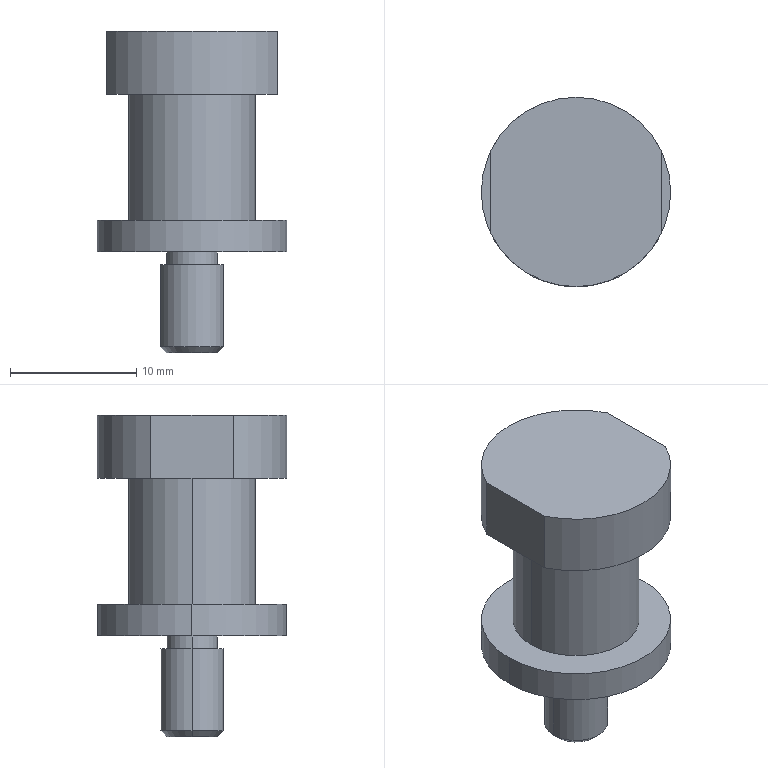Part | STEP file | PN_0036 | 1 solid | 20 faces | box 15 x 15 x 25.5 mm | volume 2226 mm3 | cylinder 10 | plane 8 | cone 2 | commonest cylinder face diameters 15 x4 4 x2 5 x2 10 x2
STEP:
#1=CARTESIAN_POINT('',(0.,0.,0.));
#2=DIRECTION('',(0.,0.,1.));
#3=DIRECTION('',(1.,0.,0.));
#4=AXIS2_PLACEMENT_3D('',#1,#2,#3);
#5=CARTESIAN_POINT('',(-2.,0.,-10.5));
#6=VERTEX_POINT('',#5);
#7=CARTESIAN_POINT('',(2.,0.,-10.5));
#8=VERTEX_POINT('',#7);
#9=CARTESIAN_POINT('',(0.,0.,-10.5));
#10=DIRECTION('',(0.,0.,-1.));
#11=DIRECTION('',(-1.,0.,0.));
#12=AXIS2_PLACEMENT_3D('',#9,#10,#11);
#13=CIRCLE('',#12,2.);
#14=CARTESIAN_POINT('',(0.,0.,-10.5));
#15=DIRECTION('',(0.,0.,1.));
#16=DIRECTION('',(1.,0.,0.));
#17=AXIS2_PLACEMENT_3D('',#14,#15,#16);
#18=CONICAL_SURFACE('',#17,2.,0.7854);
#19=CARTESIAN_POINT('',(3.142,0.));
#20=DIRECTION('',(-1.,0.));
#21=VECTOR('',#20,1.);
#22=LINE('',#19,#21);
#23=(GEOMETRIC_REPRESENTATION_CONTEXT(2)PARAMETRIC_REPRESENTATION_CONTEXT()REPRESENTATION_CONTEXT('',''));
#24=DEFINITIONAL_REPRESENTATION('',(#22),#23);
#25=PCURVE('',#18,#24);
#26=CARTESIAN_POINT('',(0.,0.,-10.5));
#27=DIRECTION('',(0.,0.,-1.));
#28=DIRECTION('',(-1.,0.,0.));
#29=AXIS2_PLACEMENT_3D('',#26,#27,#28);
#30=PLANE('',#29);
#31=CARTESIAN_POINT('',(0.,0.));
#32=DIRECTION('',(1.,0.));
#33=AXIS2_PLACEMENT_2D('',#31,#32);
#34=CIRCLE('',#33,2.);
#35=(GEOMETRIC_REPRESENTATION_CONTEXT(2)PARAMETRIC_REPRESENTATION_CONTEXT()REPRESENTATION_CONTEXT('',''));
#36=DEFINITIONAL_REPRESENTATION('',(#34),#35);
#37=PCURVE('',#30,#36);
#38=SURFACE_CURVE('',#13,(#25,#37),.PCURVE_S1.);
#39=EDGE_CURVE('',#6,#8,#38,.T.);
#40=ORIENTED_EDGE('',*,*,#39,.F.);
#41=CARTESIAN_POINT('',(-2.5,0.,-10.));
#42=VERTEX_POINT('',#41);
#43=CARTESIAN_POINT('',(-2.,0.,-10.5));
#44=DIRECTION('',(-0.7071,0.,0.7071));
#45=VECTOR('',#44,1.);
#46=LINE('',#43,#45);
#47=CARTESIAN_POINT('',(3.142,0.));
#48=DIRECTION('',(0.,1.));
#49=VECTOR('',#48,1.);
#50=LINE('',#47,#49);
#51=(GEOMETRIC_REPRESENTATION_CONTEXT(2)PARAMETRIC_REPRESENTATION_CONTEXT()REPRESENTATION_CONTEXT('',''));
#52=DEFINITIONAL_REPRESENTATION('',(#50),#51);
#53=PCURVE('',#18,#52);
#54=CARTESIAN_POINT('',(0.,0.,-10.5));
#55=DIRECTION('',(0.,0.,1.));
#56=DIRECTION('',(1.,0.,0.));
#57=AXIS2_PLACEMENT_3D('',#54,#55,#56);
#58=CONICAL_SURFACE('',#57,2.,0.7854);
#59=CARTESIAN_POINT('',(3.142,0.));
#60=DIRECTION('',(0.,1.));
#61=VECTOR('',#60,1.);
#62=LINE('',#59,#61);
#63=(GEOMETRIC_REPRESENTATION_CONTEXT(2)PARAMETRIC_REPRESENTATION_CONTEXT()REPRESENTATION_CONTEXT('',''));
#64=DEFINITIONAL_REPRESENTATION('',(#62),#63);
#65=PCURVE('',#58,#64);
#66=SURFACE_CURVE('',#46,(#53,#65),.PCURVE_S1.);
#67=EDGE_CURVE('',#6,#42,#66,.T.);
#68=ORIENTED_EDGE('',*,*,#67,.T.);
#69=CARTESIAN_POINT('',(2.5,0.,-10.));
#70=VERTEX_POINT('',#69);
#71=CARTESIAN_POINT('',(0.,0.,-10.));
#72=DIRECTION('',(0.,0.,1.));
#73=DIRECTION('',(-1.,0.,0.));
#74=AXIS2_PLACEMENT_3D('',#71,#72,#73);
#75=CIRCLE('',#74,2.5);
#76=CARTESIAN_POINT('',(-3.142,0.5));
#77=DIRECTION('',(1.,0.));
#78=VECTOR('',#77,1.);
#79=LINE('',#76,#78);
#80=(GEOMETRIC_REPRESENTATION_CONTEXT(2)PARAMETRIC_REPRESENTATION_CONTEXT()REPRESENTATION_CONTEXT('',''));
#81=DEFINITIONAL_REPRESENTATION('',(#79),#80);
#82=PCURVE('',#18,#81);
#83=CARTESIAN_POINT('',(0.,0.,-10.5));
#84=DIRECTION('',(0.,0.,1.));
#85=DIRECTION('',(1.,0.,0.));
#86=AXIS2_PLACEMENT_3D('',#83,#84,#85);
#87=CYLINDRICAL_SURFACE('',#86,2.5);
#88=CARTESIAN_POINT('',(-3.142,0.5));
#89=DIRECTION('',(1.,0.));
#90=VECTOR('',#89,1.);
#91=LINE('',#88,#90);
#92=(GEOMETRIC_REPRESENTATION_CONTEXT(2)PARAMETRIC_REPRESENTATION_CONTEXT()REPRESENTATION_CONTEXT('',''));
#93=DEFINITIONAL_REPRESENTATION('',(#91),#92);
#94=PCURVE('',#87,#93);
#95=SURFACE_CURVE('',#75,(#82,#94),.PCURVE_S1.);
#96=EDGE_CURVE('',#70,#42,#95,.T.);
#97=ORIENTED_EDGE('',*,*,#96,.F.);
#98=CARTESIAN_POINT('',(2.,0.,-10.5));
#99=DIRECTION('',(0.7071,0.,0.7071));
#100=VECTOR('',#99,1.);
#101=LINE('',#98,#100);
#102=CARTESIAN_POINT('',(0.,0.));
#103=DIRECTION('',(0.,1.));
#104=VECTOR('',#103,1.);
#105=LINE('',#102,#104);
#106=(GEOMETRIC_REPRESENTATION_CONTEXT(2)PARAMETRIC_REPRESENTATION_CONTEXT()REPRESENTATION_CONTEXT('',''));
#107=DEFINITIONAL_REPRESENTATION('',(#105),#106);
#108=PCURVE('',#18,#107);
#109=CARTESIAN_POINT('',(6.283,0.));
#110=DIRECTION('',(0.,1.));
#111=VECTOR('',#110,1.);
#112=LINE('',#109,#111);
#113=(GEOMETRIC_REPRESENTATION_CONTEXT(2)PARAMETRIC_REPRESENTATION_CONTEXT()REPRESENTATION_CONTEXT('',''));
#114=DEFINITIONAL_REPRESENTATION('',(#112),#113);
#115=PCURVE('',#58,#114);
#116=SURFACE_CURVE('',#101,(#108,#115),.PCURVE_S1.);
#117=EDGE_CURVE('',#8,#70,#116,.T.);
#118=ORIENTED_EDGE('',*,*,#117,.F.);
#119=EDGE_LOOP('',(#40,#68,#97,#118));
#120=FACE_BOUND('',#119,.T.);
#121=ADVANCED_FACE('',(#120),#18,.T.);
#122=ORIENTED_EDGE('',*,*,#96,.T.);
#123=CARTESIAN_POINT('',(-2.5,0.,-3.5));
#124=VERTEX_POINT('',#123);
#125=CARTESIAN_POINT('',(-2.5,0.,-10.5));
#126=DIRECTION('',(0.,0.,1.));
#127=VECTOR('',#126,1.);
#128=LINE('',#125,#127);
#129=CARTESIAN_POINT('',(3.142,0.));
#130=DIRECTION('',(0.,1.));
#131=VECTOR('',#130,1.);
#132=LINE('',#129,#131);
#133=(GEOMETRIC_REPRESENTATION_CONTEXT(2)PARAMETRIC_REPRESENTATION_CONTEXT()REPRESENTATION_CONTEXT('',''));
#134=DEFINITIONAL_REPRESENTATION('',(#132),#133);
#135=PCURVE('',#87,#134);
#136=CARTESIAN_POINT('',(0.,0.,-10.5));
#137=DIRECTION('',(0.,0.,1.));
#138=DIRECTION('',(1.,0.,0.));
#139=AXIS2_PLACEMENT_3D('',#136,#137,#138);
#140=CYLINDRICAL_SURFACE('',#139,2.5);
#141=CARTESIAN_POINT('',(3.142,0.));
#142=DIRECTION('',(0.,1.));
#143=VECTOR('',#142,1.);
#144=LINE('',#141,#143);
#145=(GEOMETRIC_REPRESENTATION_CONTEXT(2)PARAMETRIC_REPRESENTATION_CONTEXT()REPRESENTATION_CONTEXT('',''));
#146=DEFINITIONAL_REPRESENTATION('',(#144),#145);
#147=PCURVE('',#140,#146);
#148=SURFACE_CURVE('',#128,(#135,#147),.PCURVE_S1.);
#149=EDGE_CURVE('',#42,#124,#148,.T.);
#150=ORIENTED_EDGE('',*,*,#149,.T.);
#151=CARTESIAN_POINT('',(2.5,0.,-3.5));
#152=VERTEX_POINT('',#151);
#153=CARTESIAN_POINT('',(0.,0.,-3.5));
#154=DIRECTION('',(0.,0.,-1.));
#155=DIRECTION('',(-1.,0.,0.));
#156=AXIS2_PLACEMENT_3D('',#153,#154,#155);
#157=CIRCLE('',#156,2.5);
#158=CARTESIAN_POINT('',(3.142,7.));
#159=DIRECTION('',(-1.,0.));
#160=VECTOR('',#159,1.);
#161=LINE('',#158,#160);
#162=(GEOMETRIC_REPRESENTATION_CONTEXT(2)PARAMETRIC_REPRESENTATION_CONTEXT()REPRESENTATION_CONTEXT('',''));
#163=DEFINITIONAL_REPRESENTATION('',(#161),#162);
#164=PCURVE('',#87,#163);
#165=CARTESIAN_POINT('',(0.,0.,-3.5));
#166=DIRECTION('',(0.,0.,-1.));
#167=DIRECTION('',(-1.,0.,0.));
#168=AXIS2_PLACEMENT_3D('',#165,#166,#167);
#169=PLANE('',#168);
#170=CARTESIAN_POINT('',(0.,0.));
#171=DIRECTION('',(1.,0.));
#172=AXIS2_PLACEMENT_2D('',#170,#171);
#173=CIRCLE('',#172,2.5);
#174=(GEOMETRIC_REPRESENTATION_CONTEXT(2)PARAMETRIC_REPRESENTATION_CONTEXT()REPRESENTATION_CONTEXT('',''));
#175=DEFINITIONAL_REPRESENTATION('',(#173),#174);
#176=PCURVE('',#169,#175);
#177=SURFACE_CURVE('',#157,(#164,#176),.PCURVE_S1.);
#178=EDGE_CURVE('',#124,#152,#177,.T.);
#179=ORIENTED_EDGE('',*,*,#178,.T.);
#180=CARTESIAN_POINT('',(2.5,0.,-10.5));
#181=DIRECTION('',(0.,0.,1.));
#182=VECTOR('',#181,1.);
#183=LINE('',#180,#182);
#184=CARTESIAN_POINT('',(0.,0.));
#185=DIRECTION('',(0.,1.));
#186=VECTOR('',#185,1.);
#187=LINE('',#184,#186);
#188=(GEOMETRIC_REPRESENTATION_CONTEXT(2)PARAMETRIC_REPRESENTATION_CONTEXT()REPRESENTATION_CONTEXT('',''));
#189=DEFINITIONAL_REPRESENTATION('',(#187),#188);
#190=PCURVE('',#87,#189);
#191=CARTESIAN_POINT('',(6.283,0.));
#192=DIRECTION('',(0.,1.));
#193=VECTOR('',#192,1.);
#194=LINE('',#191,#193);
#195=(GEOMETRIC_REPRESENTATION_CONTEXT(2)PARAMETRIC_REPRESENTATION_CONTEXT()REPRESENTATION_CONTEXT('',''));
#196=DEFINITIONAL_REPRESENTATION('',(#194),#195);
#197=PCURVE('',#140,#196);
#198=SURFACE_CURVE('',#183,(#190,#197),.PCURVE_S1.);
#199=EDGE_CURVE('',#70,#152,#198,.T.);
#200=ORIENTED_EDGE('',*,*,#199,.F.);
#201=EDGE_LOOP('',(#122,#150,#179,#200));
#202=FACE_BOUND('',#201,.T.);
#203=ADVANCED_FACE('',(#202),#87,.T.);
#204=CARTESIAN_POINT('',(-2.,0.,-3.5));
#205=VERTEX_POINT('',#204);
#206=CARTESIAN_POINT('',(2.,0.,-3.5));
#207=VERTEX_POINT('',#206);
#208=CARTESIAN_POINT('',(0.,0.,-3.5));
#209=DIRECTION('',(0.,0.,-1.));
#210=DIRECTION('',(-1.,0.,0.));
#211=AXIS2_PLACEMENT_3D('',#208,#209,#210);
#212=CIRCLE('',#211,2.);
#213=CARTESIAN_POINT('',(0.,0.,-3.5));
#214=DIRECTION('',(0.,0.,1.));
#215=DIRECTION('',(1.,0.,0.));
#216=AXIS2_PLACEMENT_3D('',#213,#214,#215);
#217=CYLINDRICAL_SURFACE('',#216,2.);
#218=CARTESIAN_POINT('',(3.142,0.));
#219=DIRECTION('',(-1.,0.));
#220=VECTOR('',#219,1.);
#221=LINE('',#218,#220);
#222=(GEOMETRIC_REPRESENTATION_CONTEXT(2)PARAMETRIC_REPRESENTATION_CONTEXT()REPRESENTATION_CONTEXT('',''));
#223=DEFINITIONAL_REPRESENTATION('',(#221),#222);
#224=PCURVE('',#217,#223);
#225=CARTESIAN_POINT('',(0.,0.));
#226=DIRECTION('',(1.,0.));
#227=AXIS2_PLACEMENT_2D('',#225,#226);
#228=CIRCLE('',#227,2.);
#229=(GEOMETRIC_REPRESENTATION_CONTEXT(2)PARAMETRIC_REPRESENTATION_CONTEXT()REPRESENTATION_CONTEXT('',''));
#230=DEFINITIONAL_REPRESENTATION('',(#228),#229);
#231=PCURVE('',#169,#230);
#232=SURFACE_CURVE('',#212,(#224,#231),.PCURVE_S1.);
#233=EDGE_CURVE('',#205,#207,#232,.T.);
#234=ORIENTED_EDGE('',*,*,#233,.F.);
#235=CARTESIAN_POINT('',(-2.,0.,-2.5));
#236=VERTEX_POINT('',#235);
#237=CARTESIAN_POINT('',(-2.,0.,-3.5));
#238=DIRECTION('',(0.,0.,1.));
#239=VECTOR('',#238,1.);
#240=LINE('',#237,#239);
#241=CARTESIAN_POINT('',(3.142,0.));
#242=DIRECTION('',(0.,1.));
#243=VECTOR('',#242,1.);
#244=LINE('',#241,#243);
#245=(GEOMETRIC_REPRESENTATION_CONTEXT(2)PARAMETRIC_REPRESENTATION_CONTEXT()REPRESENTATION_CONTEXT('',''));
#246=DEFINITIONAL_REPRESENTATION('',(#244),#245);
#247=PCURVE('',#217,#246);
#248=CARTESIAN_POINT('',(0.,0.,-3.5));
#249=DIRECTION('',(0.,0.,1.));
#250=DIRECTION('',(1.,0.,0.));
#251=AXIS2_PLACEMENT_3D('',#248,#249,#250);
#252=CYLINDRICAL_SURFACE('',#251,2.);
#253=CARTESIAN_POINT('',(3.142,0.));
#254=DIRECTION('',(0.,1.));
#255=VECTOR('',#254,1.);
#256=LINE('',#253,#255);
#257=(GEOMETRIC_REPRESENTATION_CONTEXT(2)PARAMETRIC_REPRESENTATION_CONTEXT()REPRESENTATION_CONTEXT('',''));
#258=DEFINITIONAL_REPRESENTATION('',(#256),#257);
#259=PCURVE('',#252,#258);
#260=SURFACE_CURVE('',#240,(#247,#259),.PCURVE_S1.);
#261=EDGE_CURVE('',#205,#236,#260,.T.);
#262=ORIENTED_EDGE('',*,*,#261,.T.);
#263=CARTESIAN_POINT('',(2.,0.,-2.5));
#264=VERTEX_POINT('',#263);
#265=CARTESIAN_POINT('',(0.,0.,-2.5));
#266=DIRECTION('',(0.,0.,-1.));
#267=DIRECTION('',(-1.,0.,0.));
#268=AXIS2_PLACEMENT_3D('',#265,#266,#267);
#269=CIRCLE('',#268,2.);
#270=CARTESIAN_POINT('',(3.142,1.));
#271=DIRECTION('',(-1.,0.));
#272=VECTOR('',#271,1.);
#273=LINE('',#270,#272);
#274=(GEOMETRIC_REPRESENTATION_CONTEXT(2)PARAMETRIC_REPRESENTATION_CONTEXT()REPRESENTATION_CONTEXT('',''));
#275=DEFINITIONAL_REPRESENTATION('',(#273),#274);
#276=PCURVE('',#217,#275);
#277=CARTESIAN_POINT('',(0.,0.,-2.5));
#278=DIRECTION('',(0.,0.,-1.));
#279=DIRECTION('',(-1.,0.,0.));
#280=AXIS2_PLACEMENT_3D('',#277,#278,#279);
#281=PLANE('',#280);
#282=CARTESIAN_POINT('',(0.,0.));
#283=DIRECTION('',(1.,0.));
#284=AXIS2_PLACEMENT_2D('',#282,#283);
#285=CIRCLE('',#284,2.);
#286=(GEOMETRIC_REPRESENTATION_CONTEXT(2)PARAMETRIC_REPRESENTATION_CONTEXT()REPRESENTATION_CONTEXT('',''));
#287=DEFINITIONAL_REPRESENTATION('',(#285),#286);
#288=PCURVE('',#281,#287);
#289=SURFACE_CURVE('',#269,(#276,#288),.PCURVE_S1.);
#290=EDGE_CURVE('',#236,#264,#289,.T.);
#291=ORIENTED_EDGE('',*,*,#290,.T.);
#292=CARTESIAN_POINT('',(2.,0.,-3.5));
#293=DIRECTION('',(0.,0.,1.));
#294=VECTOR('',#293,1.);
#295=LINE('',#292,#294);
#296=CARTESIAN_POINT('',(0.,0.));
#297=DIRECTION('',(0.,1.));
#298=VECTOR('',#297,1.);
#299=LINE('',#296,#298);
#300=(GEOMETRIC_REPRESENTATION_CONTEXT(2)PARAMETRIC_REPRESENTATION_CONTEXT()REPRESENTATION_CONTEXT('',''));
#301=DEFINITIONAL_REPRESENTATION('',(#299),#300);
#302=PCURVE('',#217,#301);
#303=CARTESIAN_POINT('',(6.283,0.));
#304=DIRECTION('',(0.,1.));
#305=VECTOR('',#304,1.);
#306=LINE('',#303,#305);
#307=(GEOMETRIC_REPRESENTATION_CONTEXT(2)PARAMETRIC_REPRESENTATION_CONTEXT()REPRESENTATION_CONTEXT('',''));
#308=DEFINITIONAL_REPRESENTATION('',(#306),#307);
#309=PCURVE('',#252,#308);
#310=SURFACE_CURVE('',#295,(#302,#309),.PCURVE_S1.);
#311=EDGE_CURVE('',#207,#264,#310,.T.);
#312=ORIENTED_EDGE('',*,*,#311,.F.);
#313=EDGE_LOOP('',(#234,#262,#291,#312));
#314=FACE_BOUND('',#313,.T.);
#315=ADVANCED_FACE('',(#314),#217,.T.);
#316=CARTESIAN_POINT('',(-7.5,0.,-2.5));
#317=VERTEX_POINT('',#316);
#318=CARTESIAN_POINT('',(7.5,0.,-2.5));
#319=VERTEX_POINT('',#318);
#320=CARTESIAN_POINT('',(0.,0.,-2.5));
#321=DIRECTION('',(0.,0.,-1.));
#322=DIRECTION('',(-1.,0.,0.));
#323=AXIS2_PLACEMENT_3D('',#320,#321,#322);
#324=CIRCLE('',#323,7.5);
#325=CARTESIAN_POINT('',(0.,0.,-2.5));
#326=DIRECTION('',(0.,0.,1.));
#327=DIRECTION('',(1.,0.,0.));
#328=AXIS2_PLACEMENT_3D('',#325,#326,#327);
#329=CYLINDRICAL_SURFACE('',#328,7.5);
#330=CARTESIAN_POINT('',(3.142,0.));
#331=DIRECTION('',(-1.,0.));
#332=VECTOR('',#331,1.);
#333=LINE('',#330,#332);
#334=(GEOMETRIC_REPRESENTATION_CONTEXT(2)PARAMETRIC_REPRESENTATION_CONTEXT()REPRESENTATION_CONTEXT('',''));
#335=DEFINITIONAL_REPRESENTATION('',(#333),#334);
#336=PCURVE('',#329,#335);
#337=CARTESIAN_POINT('',(0.,0.));
#338=DIRECTION('',(1.,0.));
#339=AXIS2_PLACEMENT_2D('',#337,#338);
#340=CIRCLE('',#339,7.5);
#341=(GEOMETRIC_REPRESENTATION_CONTEXT(2)PARAMETRIC_REPRESENTATION_CONTEXT()REPRESENTATION_CONTEXT('',''));
#342=DEFINITIONAL_REPRESENTATION('',(#340),#341);
#343=PCURVE('',#281,#342);
#344=SURFACE_CURVE('',#324,(#336,#343),.PCURVE_S1.);
#345=EDGE_CURVE('',#317,#319,#344,.T.);
#346=ORIENTED_EDGE('',*,*,#345,.F.);
#347=CARTESIAN_POINT('',(-7.5,0.,0.));
#348=VERTEX_POINT('',#347);
#349=CARTESIAN_POINT('',(-7.5,0.,-2.5));
#350=DIRECTION('',(0.,0.,1.));
#351=VECTOR('',#350,1.);
#352=LINE('',#349,#351);
#353=CARTESIAN_POINT('',(3.142,0.));
#354=DIRECTION('',(0.,1.));
#355=VECTOR('',#354,1.);
#356=LINE('',#353,#355);
#357=(GEOMETRIC_REPRESENTATION_CONTEXT(2)PARAMETRIC_REPRESENTATION_CONTEXT()REPRESENTATION_CONTEXT('',''));
#358=DEFINITIONAL_REPRESENTATION('',(#356),#357);
#359=PCURVE('',#329,#358);
#360=CARTESIAN_POINT('',(0.,0.,-2.5));
#361=DIRECTION('',(0.,0.,1.));
#362=DIRECTION('',(1.,0.,0.));
#363=AXIS2_PLACEMENT_3D('',#360,#361,#362);
#364=CYLINDRICAL_SURFACE('',#363,7.5);
#365=CARTESIAN_POINT('',(3.142,0.));
#366=DIRECTION('',(0.,1.));
#367=VECTOR('',#366,1.);
#368=LINE('',#365,#367);
#369=(GEOMETRIC_REPRESENTATION_CONTEXT(2)PARAMETRIC_REPRESENTATION_CONTEXT()REPRESENTATION_CONTEXT('',''));
#370=DEFINITIONAL_REPRESENTATION('',(#368),#369);
#371=PCURVE('',#364,#370);
#372=SURFACE_CURVE('',#352,(#359,#371),.PCURVE_S1.);
#373=EDGE_CURVE('',#317,#348,#372,.T.);
#374=ORIENTED_EDGE('',*,*,#373,.T.);
#375=CARTESIAN_POINT('',(7.5,0.,0.));
#376=VERTEX_POINT('',#375);
#377=CARTESIAN_POINT('',(0.,0.,0.));
#378=DIRECTION('',(0.,0.,-1.));
#379=DIRECTION('',(-1.,0.,0.));
#380=AXIS2_PLACEMENT_3D('',#377,#378,#379);
#381=CIRCLE('',#380,7.5);
#382=CARTESIAN_POINT('',(3.142,2.5));
#383=DIRECTION('',(-1.,0.));
#384=VECTOR('',#383,1.);
#385=LINE('',#382,#384);
#386=(GEOMETRIC_REPRESENTATION_CONTEXT(2)PARAMETRIC_REPRESENTATION_CONTEXT()REPRESENTATION_CONTEXT('',''));
#387=DEFINITIONAL_REPRESENTATION('',(#385),#386);
#388=PCURVE('',#329,#387);
#389=CARTESIAN_POINT('',(0.,0.,0.));
#390=DIRECTION('',(0.,0.,-1.));
#391=DIRECTION('',(-1.,0.,0.));
#392=AXIS2_PLACEMENT_3D('',#389,#390,#391);
#393=PLANE('',#392);
#394=CARTESIAN_POINT('',(0.,0.));
#395=DIRECTION('',(1.,0.));
#396=AXIS2_PLACEMENT_2D('',#394,#395);
#397=CIRCLE('',#396,7.5);
#398=(GEOMETRIC_REPRESENTATION_CONTEXT(2)PARAMETRIC_REPRESENTATION_CONTEXT()REPRESENTATION_CONTEXT('',''));
#399=DEFINITIONAL_REPRESENTATION('',(#397),#398);
#400=PCURVE('',#393,#399);
#401=SURFACE_CURVE('',#381,(#388,#400),.PCURVE_S1.);
#402=EDGE_CURVE('',#348,#376,#401,.T.);
#403=ORIENTED_EDGE('',*,*,#402,.T.);
#404=CARTESIAN_POINT('',(7.5,0.,-2.5));
#405=DIRECTION('',(0.,0.,1.));
#406=VECTOR('',#405,1.);
#407=LINE('',#404,#406);
#408=CARTESIAN_POINT('',(0.,0.));
#409=DIRECTION('',(0.,1.));
#410=VECTOR('',#409,1.);
#411=LINE('',#408,#410);
#412=(GEOMETRIC_REPRESENTATION_CONTEXT(2)PARAMETRIC_REPRESENTATION_CONTEXT()REPRESENTATION_CONTEXT('',''));
#413=DEFINITIONAL_REPRESENTATION('',(#411),#412);
#414=PCURVE('',#329,#413);
#415=CARTESIAN_POINT('',(6.283,0.));
#416=DIRECTION('',(0.,1.));
#417=VECTOR('',#416,1.);
#418=LINE('',#415,#417);
#419=(GEOMETRIC_REPRESENTATION_CONTEXT(2)PARAMETRIC_REPRESENTATION_CONTEXT()REPRESENTATION_CONTEXT('',''));
#420=DEFINITIONAL_REPRESENTATION('',(#418),#419);
#421=PCURVE('',#364,#420);
#422=SURFACE_CURVE('',#407,(#414,#421),.PCURVE_S1.);
#423=EDGE_CURVE('',#319,#376,#422,.T.);
#424=ORIENTED_EDGE('',*,*,#423,.F.);
#425=EDGE_LOOP('',(#346,#374,#403,#424));
#426=FACE_BOUND('',#425,.T.);
#427=ADVANCED_FACE('',(#426),#329,.T.);
#428=CARTESIAN_POINT('',(5.,0.,10.));
#429=VERTEX_POINT('',#428);
#430=CARTESIAN_POINT('',(-5.,0.,10.));
#431=VERTEX_POINT('',#430);
#432=CARTESIAN_POINT('',(0.,0.,10.));
#433=DIRECTION('',(0.,0.,1.));
#434=DIRECTION('',(1.,0.,0.));
#435=AXIS2_PLACEMENT_3D('',#432,#433,#434);
#436=CIRCLE('',#435,5.);
#437=CARTESIAN_POINT('',(0.,0.,10.));
#438=DIRECTION('',(0.,0.,-1.));
#439=DIRECTION('',(-1.,0.,0.));
#440=AXIS2_PLACEMENT_3D('',#437,#438,#439);
#441=CYLINDRICAL_SURFACE('',#440,5.);
#442=CARTESIAN_POINT('',(3.142,0.));
#443=DIRECTION('',(-1.,0.));
#444=VECTOR('',#443,1.);
#445=LINE('',#442,#444);
#446=(GEOMETRIC_REPRESENTATION_CONTEXT(2)PARAMETRIC_REPRESENTATION_CONTEXT()REPRESENTATION_CONTEXT('',''));
#447=DEFINITIONAL_REPRESENTATION('',(#445),#446);
#448=PCURVE('',#441,#447);
#449=CARTESIAN_POINT('',(0.,0.,10.));
#450=DIRECTION('',(0.,0.,1.));
#451=DIRECTION('',(1.,0.,0.));
#452=AXIS2_PLACEMENT_3D('',#449,#450,#451);
#453=PLANE('',#452);
#454=CARTESIAN_POINT('',(0.,0.));
#455=DIRECTION('',(1.,0.));
#456=AXIS2_PLACEMENT_2D('',#454,#455);
#457=CIRCLE('',#456,5.);
#458=(GEOMETRIC_REPRESENTATION_CONTEXT(2)PARAMETRIC_REPRESENTATION_CONTEXT()REPRESENTATION_CONTEXT('',''));
#459=DEFINITIONAL_REPRESENTATION('',(#457),#458);
#460=PCURVE('',#453,#459);
#461=SURFACE_CURVE('',#436,(#448,#460),.PCURVE_S1.);
#462=EDGE_CURVE('',#429,#431,#461,.T.);
#463=ORIENTED_EDGE('',*,*,#462,.F.);
#464=CARTESIAN_POINT('',(5.,0.,0.));
#465=VERTEX_POINT('',#464);
#466=CARTESIAN_POINT('',(5.,0.,10.));
#467=DIRECTION('',(0.,0.,-1.));
#468=VECTOR('',#467,1.);
#469=LINE('',#466,#468);
#470=CARTESIAN_POINT('',(3.142,0.));
#471=DIRECTION('',(0.,1.));
#472=VECTOR('',#471,1.);
#473=LINE('',#470,#472);
#474=(GEOMETRIC_REPRESENTATION_CONTEXT(2)PARAMETRIC_REPRESENTATION_CONTEXT()REPRESENTATION_CONTEXT('',''));
#475=DEFINITIONAL_REPRESENTATION('',(#473),#474);
#476=PCURVE('',#441,#475);
#477=CARTESIAN_POINT('',(0.,0.,10.));
#478=DIRECTION('',(0.,0.,-1.));
#479=DIRECTION('',(-1.,0.,0.));
#480=AXIS2_PLACEMENT_3D('',#477,#478,#479);
#481=CYLINDRICAL_SURFACE('',#480,5.);
#482=CARTESIAN_POINT('',(3.142,0.));
#483=DIRECTION('',(0.,1.));
#484=VECTOR('',#483,1.);
#485=LINE('',#482,#484);
#486=(GEOMETRIC_REPRESENTATION_CONTEXT(2)PARAMETRIC_REPRESENTATION_CONTEXT()REPRESENTATION_CONTEXT('',''));
#487=DEFINITIONAL_REPRESENTATION('',(#485),#486);
#488=PCURVE('',#481,#487);
#489=SURFACE_CURVE('',#469,(#476,#488),.PCURVE_S1.);
#490=EDGE_CURVE('',#429,#465,#489,.T.);
#491=ORIENTED_EDGE('',*,*,#490,.T.);
#492=CARTESIAN_POINT('',(-5.,0.,0.));
#493=VERTEX_POINT('',#492);
#494=CARTESIAN_POINT('',(0.,0.,0.));
#495=DIRECTION('',(0.,0.,-1.));
#496=DIRECTION('',(-1.,0.,0.));
#497=AXIS2_PLACEMENT_3D('',#494,#495,#496);
#498=CIRCLE('',#497,5.);
#499=CARTESIAN_POINT('',(0.,10.));
#500=DIRECTION('',(1.,0.));
#501=VECTOR('',#500,1.);
#502=LINE('',#499,#501);
#503=(GEOMETRIC_REPRESENTATION_CONTEXT(2)PARAMETRIC_REPRESENTATION_CONTEXT()REPRESENTATION_CONTEXT('',''));
#504=DEFINITIONAL_REPRESENTATION('',(#502),#503);
#505=PCURVE('',#441,#504);
#506=CARTESIAN_POINT('',(0.,0.));
#507=DIRECTION('',(1.,0.));
#508=AXIS2_PLACEMENT_2D('',#506,#507);
#509=CIRCLE('',#508,5.);
#510=(GEOMETRIC_REPRESENTATION_CONTEXT(2)PARAMETRIC_REPRESENTATION_CONTEXT()REPRESENTATION_CONTEXT('',''));
#511=DEFINITIONAL_REPRESENTATION('',(#509),#510);
#512=PCURVE('',#393,#511);
#513=SURFACE_CURVE('',#498,(#505,#512),.PCURVE_S1.);
#514=EDGE_CURVE('',#493,#465,#513,.T.);
#515=ORIENTED_EDGE('',*,*,#514,.F.);
#516=CARTESIAN_POINT('',(-5.,0.,10.));
#517=DIRECTION('',(0.,0.,-1.));
#518=VECTOR('',#517,1.);
#519=LINE('',#516,#518);
#520=CARTESIAN_POINT('',(0.,0.));
#521=DIRECTION('',(0.,1.));
#522=VECTOR('',#521,1.);
#523=LINE('',#520,#522);
#524=(GEOMETRIC_REPRESENTATION_CONTEXT(2)PARAMETRIC_REPRESENTATION_CONTEXT()REPRESENTATION_CONTEXT('',''));
#525=DEFINITIONAL_REPRESENTATION('',(#523),#524);
#526=PCURVE('',#441,#525);
#527=CARTESIAN_POINT('',(6.283,0.));
#528=DIRECTION('',(0.,1.));
#529=VECTOR('',#528,1.);
#530=LINE('',#527,#529);
#531=(GEOMETRIC_REPRESENTATION_CONTEXT(2)PARAMETRIC_REPRESENTATION_CONTEXT()REPRESENTATION_CONTEXT('',''));
#532=DEFINITIONAL_REPRESENTATION('',(#530),#531);
#533=PCURVE('',#481,#532);
#534=SURFACE_CURVE('',#519,(#526,#533),.PCURVE_S1.);
#535=EDGE_CURVE('',#431,#493,#534,.T.);
#536=ORIENTED_EDGE('',*,*,#535,.F.);
#537=EDGE_LOOP('',(#463,#491,#515,#536));
#538=FACE_BOUND('',#537,.T.);
#539=ADVANCED_FACE('',(#538),#441,.T.);
#540=CARTESIAN_POINT('',(0.,0.,-2.5));
#541=DIRECTION('',(0.,0.,-1.));
#542=DIRECTION('',(-1.,0.,0.));
#543=AXIS2_PLACEMENT_3D('',#540,#541,#542);
#544=CIRCLE('',#543,7.5);
#545=CARTESIAN_POINT('',(0.,0.));
#546=DIRECTION('',(1.,0.));
#547=AXIS2_PLACEMENT_2D('',#545,#546);
#548=CIRCLE('',#547,7.5);
#549=(GEOMETRIC_REPRESENTATION_CONTEXT(2)PARAMETRIC_REPRESENTATION_CONTEXT()REPRESENTATION_CONTEXT('',''));
#550=DEFINITIONAL_REPRESENTATION('',(#548),#549);
#551=PCURVE('',#281,#550);
#552=CARTESIAN_POINT('',(9.425,0.));
#553=DIRECTION('',(-1.,0.));
#554=VECTOR('',#553,1.);
#555=LINE('',#552,#554);
#556=(GEOMETRIC_REPRESENTATION_CONTEXT(2)PARAMETRIC_REPRESENTATION_CONTEXT()REPRESENTATION_CONTEXT('',''));
#557=DEFINITIONAL_REPRESENTATION('',(#555),#556);
#558=PCURVE('',#364,#557);
#559=SURFACE_CURVE('',#544,(#551,#558),.PCURVE_S1.);
#560=EDGE_CURVE('',#319,#317,#559,.T.);
#561=ORIENTED_EDGE('',*,*,#560,.T.);
#562=ORIENTED_EDGE('',*,*,#345,.T.);
#563=EDGE_LOOP('',(#561,#562));
#564=FACE_BOUND('',#563,.T.);
#565=CARTESIAN_POINT('',(0.,0.,-2.5));
#566=DIRECTION('',(0.,0.,-1.));
#567=DIRECTION('',(-1.,0.,0.));
#568=AXIS2_PLACEMENT_3D('',#565,#566,#567);
#569=CIRCLE('',#568,2.);
#570=CARTESIAN_POINT('',(0.,0.));
#571=DIRECTION('',(1.,0.));
#572=AXIS2_PLACEMENT_2D('',#570,#571);
#573=CIRCLE('',#572,2.);
#574=(GEOMETRIC_REPRESENTATION_CONTEXT(2)PARAMETRIC_REPRESENTATION_CONTEXT()REPRESENTATION_CONTEXT('',''));
#575=DEFINITIONAL_REPRESENTATION('',(#573),#574);
#576=PCURVE('',#281,#575);
#577=CARTESIAN_POINT('',(9.425,1.));
#578=DIRECTION('',(-1.,0.));
#579=VECTOR('',#578,1.);
#580=LINE('',#577,#579);
#581=(GEOMETRIC_REPRESENTATION_CONTEXT(2)PARAMETRIC_REPRESENTATION_CONTEXT()REPRESENTATION_CONTEXT('',''));
#582=DEFINITIONAL_REPRESENTATION('',(#580),#581);
#583=PCURVE('',#252,#582);
#584=SURFACE_CURVE('',#569,(#576,#583),.PCURVE_S1.);
#585=EDGE_CURVE('',#264,#236,#584,.T.);
#586=ORIENTED_EDGE('',*,*,#585,.F.);
#587=ORIENTED_EDGE('',*,*,#290,.F.);
#588=EDGE_LOOP('',(#586,#587));
#589=FACE_BOUND('',#588,.T.);
#590=ADVANCED_FACE('',(#564,#589),#281,.T.);
#591=CARTESIAN_POINT('',(6.75,3.269,15.));
#592=VERTEX_POINT('',#591);
#593=CARTESIAN_POINT('',(-6.75,3.269,15.));
#594=VERTEX_POINT('',#593);
#595=CARTESIAN_POINT('',(0.,0.,15.));
#596=DIRECTION('',(0.,0.,1.));
#597=DIRECTION('',(1.,0.,0.));
#598=AXIS2_PLACEMENT_3D('',#595,#596,#597);
#599=CIRCLE('',#598,7.5);
#600=CARTESIAN_POINT('',(0.,0.,15.));
#601=DIRECTION('',(0.,0.,-1.));
#602=DIRECTION('',(-1.,0.,0.));
#603=AXIS2_PLACEMENT_3D('',#600,#601,#602);
#604=CYLINDRICAL_SURFACE('',#603,7.5);
#605=CARTESIAN_POINT('',(3.142,0.));
#606=DIRECTION('',(-1.,0.));
#607=VECTOR('',#606,1.);
#608=LINE('',#605,#607);
#609=(GEOMETRIC_REPRESENTATION_CONTEXT(2)PARAMETRIC_REPRESENTATION_CONTEXT()REPRESENTATION_CONTEXT('',''));
#610=DEFINITIONAL_REPRESENTATION('',(#608),#609);
#611=PCURVE('',#604,#610);
#612=CARTESIAN_POINT('',(0.,0.,15.));
#613=DIRECTION('',(0.,0.,1.));
#614=DIRECTION('',(1.,0.,0.));
#615=AXIS2_PLACEMENT_3D('',#612,#613,#614);
#616=PLANE('',#615);
#617=CARTESIAN_POINT('',(0.,0.));
#618=DIRECTION('',(1.,0.));
#619=AXIS2_PLACEMENT_2D('',#617,#618);
#620=CIRCLE('',#619,7.5);
#621=(GEOMETRIC_REPRESENTATION_CONTEXT(2)PARAMETRIC_REPRESENTATION_CONTEXT()REPRESENTATION_CONTEXT('',''));
#622=DEFINITIONAL_REPRESENTATION('',(#620),#621);
#623=PCURVE('',#616,#622);
#624=SURFACE_CURVE('',#599,(#611,#623),.PCURVE_S1.);
#625=EDGE_CURVE('',#592,#594,#624,.T.);
#626=ORIENTED_EDGE('',*,*,#625,.F.);
#627=CARTESIAN_POINT('',(6.75,3.269,10.));
#628=VERTEX_POINT('',#627);
#629=CARTESIAN_POINT('',(6.75,3.269,0.));
#630=DIRECTION('',(0.,0.,1.));
#631=VECTOR('',#630,1.);
#632=LINE('',#629,#631);
#633=CARTESIAN_POINT('',(2.691,15.));
#634=DIRECTION('',(0.,-1.));
#635=VECTOR('',#634,1.);
#636=LINE('',#633,#635);
#637=(GEOMETRIC_REPRESENTATION_CONTEXT(2)PARAMETRIC_REPRESENTATION_CONTEXT()REPRESENTATION_CONTEXT('',''));
#638=DEFINITIONAL_REPRESENTATION('',(#636),#637);
#639=PCURVE('',#604,#638);
#640=CARTESIAN_POINT('',(6.75,-3.269,0.));
#641=DIRECTION('',(-1.,0.,0.));
#642=DIRECTION('',(0.,0.,1.));
#643=AXIS2_PLACEMENT_3D('',#640,#641,#642);
#644=PLANE('',#643);
#645=CARTESIAN_POINT('',(0.,6.538));
#646=DIRECTION('',(1.,0.));
#647=VECTOR('',#646,1.);
#648=LINE('',#645,#647);
#649=(GEOMETRIC_REPRESENTATION_CONTEXT(2)PARAMETRIC_REPRESENTATION_CONTEXT()REPRESENTATION_CONTEXT('',''));
#650=DEFINITIONAL_REPRESENTATION('',(#648),#649);
#651=PCURVE('',#644,#650);
#652=SURFACE_CURVE('',#632,(#639,#651),.PCURVE_S1.);
#653=EDGE_CURVE('',#628,#592,#652,.T.);
#654=ORIENTED_EDGE('',*,*,#653,.F.);
#655=CARTESIAN_POINT('',(-6.75,3.269,10.));
#656=VERTEX_POINT('',#655);
#657=CARTESIAN_POINT('',(0.,0.,10.));
#658=DIRECTION('',(0.,0.,1.));
#659=DIRECTION('',(1.,0.,0.));
#660=AXIS2_PLACEMENT_3D('',#657,#658,#659);
#661=CIRCLE('',#660,7.5);
#662=CARTESIAN_POINT('',(3.142,5.));
#663=DIRECTION('',(-1.,0.));
#664=VECTOR('',#663,1.);
#665=LINE('',#662,#664);
#666=(GEOMETRIC_REPRESENTATION_CONTEXT(2)PARAMETRIC_REPRESENTATION_CONTEXT()REPRESENTATION_CONTEXT('',''));
#667=DEFINITIONAL_REPRESENTATION('',(#665),#666);
#668=PCURVE('',#604,#667);
#669=CARTESIAN_POINT('',(0.,0.));
#670=DIRECTION('',(1.,0.));
#671=AXIS2_PLACEMENT_2D('',#669,#670);
#672=CIRCLE('',#671,7.5);
#673=(GEOMETRIC_REPRESENTATION_CONTEXT(2)PARAMETRIC_REPRESENTATION_CONTEXT()REPRESENTATION_CONTEXT('',''));
#674=DEFINITIONAL_REPRESENTATION('',(#672),#673);
#675=PCURVE('',#453,#674);
#676=SURFACE_CURVE('',#661,(#668,#675),.PCURVE_S1.);
#677=EDGE_CURVE('',#628,#656,#676,.T.);
#678=ORIENTED_EDGE('',*,*,#677,.T.);
#679=CARTESIAN_POINT('',(-6.75,3.269,0.));
#680=DIRECTION('',(0.,0.,1.));
#681=VECTOR('',#680,1.);
#682=LINE('',#679,#681);
#683=CARTESIAN_POINT('',(0.451,15.));
#684=DIRECTION('',(0.,-1.));
#685=VECTOR('',#684,1.);
#686=LINE('',#683,#685);
#687=(GEOMETRIC_REPRESENTATION_CONTEXT(2)PARAMETRIC_REPRESENTATION_CONTEXT()REPRESENTATION_CONTEXT('',''));
#688=DEFINITIONAL_REPRESENTATION('',(#686),#687);
#689=PCURVE('',#604,#688);
#690=CARTESIAN_POINT('',(-6.75,3.269,0.));
#691=DIRECTION('',(1.,0.,0.));
#692=DIRECTION('',(0.,0.,-1.));
#693=AXIS2_PLACEMENT_3D('',#690,#691,#692);
#694=PLANE('',#693);
#695=CARTESIAN_POINT('',(0.,0.));
#696=DIRECTION('',(-1.,0.));
#697=VECTOR('',#696,1.);
#698=LINE('',#695,#697);
#699=(GEOMETRIC_REPRESENTATION_CONTEXT(2)PARAMETRIC_REPRESENTATION_CONTEXT()REPRESENTATION_CONTEXT('',''));
#700=DEFINITIONAL_REPRESENTATION('',(#698),#699);
#701=PCURVE('',#694,#700);
#702=SURFACE_CURVE('',#682,(#689,#701),.PCURVE_S1.);
#703=EDGE_CURVE('',#656,#594,#702,.T.);
#704=ORIENTED_EDGE('',*,*,#703,.T.);
#705=EDGE_LOOP('',(#626,#654,#678,#704));
#706=FACE_BOUND('',#705,.T.);
#707=ADVANCED_FACE('',(#706),#604,.T.);
#708=ORIENTED_EDGE('',*,*,#490,.F.);
#709=CARTESIAN_POINT('',(0.,0.,10.));
#710=DIRECTION('',(0.,0.,1.));
#711=DIRECTION('',(1.,0.,0.));
#712=AXIS2_PLACEMENT_3D('',#709,#710,#711);
#713=CIRCLE('',#712,5.);
#714=CARTESIAN_POINT('',(9.425,0.));
#715=DIRECTION('',(-1.,0.));
#716=VECTOR('',#715,1.);
#717=LINE('',#714,#716);
#718=(GEOMETRIC_REPRESENTATION_CONTEXT(2)PARAMETRIC_REPRESENTATION_CONTEXT()REPRESENTATION_CONTEXT('',''));
#719=DEFINITIONAL_REPRESENTATION('',(#717),#718);
#720=PCURVE('',#481,#719);
#721=CARTESIAN_POINT('',(0.,0.));
#722=DIRECTION('',(1.,0.));
#723=AXIS2_PLACEMENT_2D('',#721,#722);
#724=CIRCLE('',#723,5.);
#725=(GEOMETRIC_REPRESENTATION_CONTEXT(2)PARAMETRIC_REPRESENTATION_CONTEXT()REPRESENTATION_CONTEXT('',''));
#726=DEFINITIONAL_REPRESENTATION('',(#724),#725);
#727=PCURVE('',#453,#726);
#728=SURFACE_CURVE('',#713,(#720,#727),.PCURVE_S1.);
#729=EDGE_CURVE('',#431,#429,#728,.T.);
#730=ORIENTED_EDGE('',*,*,#729,.F.);
#731=ORIENTED_EDGE('',*,*,#535,.T.);
#732=CARTESIAN_POINT('',(0.,0.,0.));
#733=DIRECTION('',(0.,0.,-1.));
#734=DIRECTION('',(-1.,0.,0.));
#735=AXIS2_PLACEMENT_3D('',#732,#733,#734);
#736=CIRCLE('',#735,5.);
#737=CARTESIAN_POINT('',(0.,10.));
#738=DIRECTION('',(1.,0.));
#739=VECTOR('',#738,1.);
#740=LINE('',#737,#739);
#741=(GEOMETRIC_REPRESENTATION_CONTEXT(2)PARAMETRIC_REPRESENTATION_CONTEXT()REPRESENTATION_CONTEXT('',''));
#742=DEFINITIONAL_REPRESENTATION('',(#740),#741);
#743=PCURVE('',#481,#742);
#744=CARTESIAN_POINT('',(0.,0.));
#745=DIRECTION('',(1.,0.));
#746=AXIS2_PLACEMENT_2D('',#744,#745);
#747=CIRCLE('',#746,5.);
#748=(GEOMETRIC_REPRESENTATION_CONTEXT(2)PARAMETRIC_REPRESENTATION_CONTEXT()REPRESENTATION_CONTEXT('',''));
#749=DEFINITIONAL_REPRESENTATION('',(#747),#748);
#750=PCURVE('',#393,#749);
#751=SURFACE_CURVE('',#736,(#743,#750),.PCURVE_S1.);
#752=EDGE_CURVE('',#465,#493,#751,.T.);
#753=ORIENTED_EDGE('',*,*,#752,.F.);
#754=EDGE_LOOP('',(#708,#730,#731,#753));
#755=FACE_BOUND('',#754,.T.);
#756=ADVANCED_FACE('',(#755),#481,.T.);
#757=ORIENTED_EDGE('',*,*,#677,.F.);
#758=CARTESIAN_POINT('',(6.75,-3.269,10.));
#759=VERTEX_POINT('',#758);
#760=CARTESIAN_POINT('',(6.75,0.,10.));
#761=DIRECTION('',(0.,-1.,0.));
#762=VECTOR('',#761,1.);
#763=LINE('',#760,#762);
#764=CARTESIAN_POINT('',(6.75,0.));
#765=DIRECTION('',(0.,-1.));
#766=VECTOR('',#765,1.);
#767=LINE('',#764,#766);
#768=(GEOMETRIC_REPRESENTATION_CONTEXT(2)PARAMETRIC_REPRESENTATION_CONTEXT()REPRESENTATION_CONTEXT('',''));
#769=DEFINITIONAL_REPRESENTATION('',(#767),#768);
#770=PCURVE('',#453,#769);
#771=CARTESIAN_POINT('',(10.,3.269));
#772=DIRECTION('',(0.,-1.));
#773=VECTOR('',#772,1.);
#774=LINE('',#771,#773);
#775=(GEOMETRIC_REPRESENTATION_CONTEXT(2)PARAMETRIC_REPRESENTATION_CONTEXT()REPRESENTATION_CONTEXT('',''));
#776=DEFINITIONAL_REPRESENTATION('',(#774),#775);
#777=PCURVE('',#644,#776);
#778=SURFACE_CURVE('',#763,(#770,#777),.PCURVE_S1.);
#779=EDGE_CURVE('',#628,#759,#778,.T.);
#780=ORIENTED_EDGE('',*,*,#779,.T.);
#781=CARTESIAN_POINT('',(-6.75,-3.269,10.));
#782=VERTEX_POINT('',#781);
#783=CARTESIAN_POINT('',(0.,0.,10.));
#784=DIRECTION('',(0.,0.,1.));
#785=DIRECTION('',(1.,0.,0.));
#786=AXIS2_PLACEMENT_3D('',#783,#784,#785);
#787=CIRCLE('',#786,7.5);
#788=CARTESIAN_POINT('',(0.,0.));
#789=DIRECTION('',(1.,0.));
#790=AXIS2_PLACEMENT_2D('',#788,#789);
#791=CIRCLE('',#790,7.5);
#792=(GEOMETRIC_REPRESENTATION_CONTEXT(2)PARAMETRIC_REPRESENTATION_CONTEXT()REPRESENTATION_CONTEXT('',''));
#793=DEFINITIONAL_REPRESENTATION('',(#791),#792);
#794=PCURVE('',#453,#793);
#795=CARTESIAN_POINT('',(0.,0.,15.));
#796=DIRECTION('',(0.,0.,-1.));
#797=DIRECTION('',(-1.,0.,0.));
#798=AXIS2_PLACEMENT_3D('',#795,#796,#797);
#799=CYLINDRICAL_SURFACE('',#798,7.5);
#800=CARTESIAN_POINT('',(9.425,5.));
#801=DIRECTION('',(-1.,0.));
#802=VECTOR('',#801,1.);
#803=LINE('',#800,#802);
#804=(GEOMETRIC_REPRESENTATION_CONTEXT(2)PARAMETRIC_REPRESENTATION_CONTEXT()REPRESENTATION_CONTEXT('',''));
#805=DEFINITIONAL_REPRESENTATION('',(#803),#804);
#806=PCURVE('',#799,#805);
#807=SURFACE_CURVE('',#787,(#794,#806),.PCURVE_S1.);
#808=EDGE_CURVE('',#782,#759,#807,.T.);
#809=ORIENTED_EDGE('',*,*,#808,.F.);
#810=CARTESIAN_POINT('',(-6.75,0.,10.));
#811=DIRECTION('',(0.,1.,0.));
#812=VECTOR('',#811,1.);
#813=LINE('',#810,#812);
#814=CARTESIAN_POINT('',(-6.75,0.));
#815=DIRECTION('',(0.,1.));
#816=VECTOR('',#815,1.);
#817=LINE('',#814,#816);
#818=(GEOMETRIC_REPRESENTATION_CONTEXT(2)PARAMETRIC_REPRESENTATION_CONTEXT()REPRESENTATION_CONTEXT('',''));
#819=DEFINITIONAL_REPRESENTATION('',(#817),#818);
#820=PCURVE('',#453,#819);
#821=CARTESIAN_POINT('',(-10.,-3.269));
#822=DIRECTION('',(0.,1.));
#823=VECTOR('',#822,1.);
#824=LINE('',#821,#823);
#825=(GEOMETRIC_REPRESENTATION_CONTEXT(2)PARAMETRIC_REPRESENTATION_CONTEXT()REPRESENTATION_CONTEXT('',''));
#826=DEFINITIONAL_REPRESENTATION('',(#824),#825);
#827=PCURVE('',#694,#826);
#828=SURFACE_CURVE('',#813,(#820,#827),.PCURVE_S1.);
#829=EDGE_CURVE('',#782,#656,#828,.T.);
#830=ORIENTED_EDGE('',*,*,#829,.T.);
#831=EDGE_LOOP('',(#757,#780,#809,#830));
#832=FACE_BOUND('',#831,.T.);
#833=ORIENTED_EDGE('',*,*,#729,.T.);
#834=ORIENTED_EDGE('',*,*,#462,.T.);
#835=EDGE_LOOP('',(#833,#834));
#836=FACE_BOUND('',#835,.T.);
#837=ADVANCED_FACE('',(#832,#836),#453,.F.);
#838=ORIENTED_EDGE('',*,*,#808,.T.);
#839=CARTESIAN_POINT('',(6.75,-3.269,15.));
#840=VERTEX_POINT('',#839);
#841=CARTESIAN_POINT('',(6.75,-3.269,0.));
#842=DIRECTION('',(0.,0.,1.));
#843=VECTOR('',#842,1.);
#844=LINE('',#841,#843);
#845=CARTESIAN_POINT('',(3.593,15.));
#846=DIRECTION('',(0.,-1.));
#847=VECTOR('',#846,1.);
#848=LINE('',#845,#847);
#849=(GEOMETRIC_REPRESENTATION_CONTEXT(2)PARAMETRIC_REPRESENTATION_CONTEXT()REPRESENTATION_CONTEXT('',''));
#850=DEFINITIONAL_REPRESENTATION('',(#848),#849);
#851=PCURVE('',#799,#850);
#852=CARTESIAN_POINT('',(0.,0.));
#853=DIRECTION('',(1.,0.));
#854=VECTOR('',#853,1.);
#855=LINE('',#852,#854);
#856=(GEOMETRIC_REPRESENTATION_CONTEXT(2)PARAMETRIC_REPRESENTATION_CONTEXT()REPRESENTATION_CONTEXT('',''));
#857=DEFINITIONAL_REPRESENTATION('',(#855),#856);
#858=PCURVE('',#644,#857);
#859=SURFACE_CURVE('',#844,(#851,#858),.PCURVE_S1.);
#860=EDGE_CURVE('',#759,#840,#859,.T.);
#861=ORIENTED_EDGE('',*,*,#860,.T.);
#862=CARTESIAN_POINT('',(-6.75,-3.269,15.));
#863=VERTEX_POINT('',#862);
#864=CARTESIAN_POINT('',(0.,0.,15.));
#865=DIRECTION('',(0.,0.,1.));
#866=DIRECTION('',(1.,0.,0.));
#867=AXIS2_PLACEMENT_3D('',#864,#865,#866);
#868=CIRCLE('',#867,7.5);
#869=CARTESIAN_POINT('',(9.425,0.));
#870=DIRECTION('',(-1.,0.));
#871=VECTOR('',#870,1.);
#872=LINE('',#869,#871);
#873=(GEOMETRIC_REPRESENTATION_CONTEXT(2)PARAMETRIC_REPRESENTATION_CONTEXT()REPRESENTATION_CONTEXT('',''));
#874=DEFINITIONAL_REPRESENTATION('',(#872),#873);
#875=PCURVE('',#799,#874);
#876=CARTESIAN_POINT('',(0.,0.));
#877=DIRECTION('',(1.,0.));
#878=AXIS2_PLACEMENT_2D('',#876,#877);
#879=CIRCLE('',#878,7.5);
#880=(GEOMETRIC_REPRESENTATION_CONTEXT(2)PARAMETRIC_REPRESENTATION_CONTEXT()REPRESENTATION_CONTEXT('',''));
#881=DEFINITIONAL_REPRESENTATION('',(#879),#880);
#882=PCURVE('',#616,#881);
#883=SURFACE_CURVE('',#868,(#875,#882),.PCURVE_S1.);
#884=EDGE_CURVE('',#863,#840,#883,.T.);
#885=ORIENTED_EDGE('',*,*,#884,.F.);
#886=CARTESIAN_POINT('',(-6.75,-3.269,0.));
#887=DIRECTION('',(0.,0.,1.));
#888=VECTOR('',#887,1.);
#889=LINE('',#886,#888);
#890=CARTESIAN_POINT('',(5.832,15.));
#891=DIRECTION('',(0.,-1.));
#892=VECTOR('',#891,1.);
#893=LINE('',#890,#892);
#894=(GEOMETRIC_REPRESENTATION_CONTEXT(2)PARAMETRIC_REPRESENTATION_CONTEXT()REPRESENTATION_CONTEXT('',''));
#895=DEFINITIONAL_REPRESENTATION('',(#893),#894);
#896=PCURVE('',#799,#895);
#897=CARTESIAN_POINT('',(0.,-6.538));
#898=DIRECTION('',(-1.,0.));
#899=VECTOR('',#898,1.);
#900=LINE('',#897,#899);
#901=(GEOMETRIC_REPRESENTATION_CONTEXT(2)PARAMETRIC_REPRESENTATION_CONTEXT()REPRESENTATION_CONTEXT('',''));
#902=DEFINITIONAL_REPRESENTATION('',(#900),#901);
#903=PCURVE('',#694,#902);
#904=SURFACE_CURVE('',#889,(#896,#903),.PCURVE_S1.);
#905=EDGE_CURVE('',#782,#863,#904,.T.);
#906=ORIENTED_EDGE('',*,*,#905,.F.);
#907=EDGE_LOOP('',(#838,#861,#885,#906));
#908=FACE_BOUND('',#907,.T.);
#909=ADVANCED_FACE('',(#908),#799,.T.);
#910=CARTESIAN_POINT('',(6.75,-3.269,15.));
#911=DIRECTION('',(0.,-1.,0.));
#912=VECTOR('',#911,1.);
#913=LINE('',#910,#912);
#914=CARTESIAN_POINT('',(6.75,-3.269));
#915=DIRECTION('',(0.,-1.));
#916=VECTOR('',#915,1.);
#917=LINE('',#914,#916);
#918=(GEOMETRIC_REPRESENTATION_CONTEXT(2)PARAMETRIC_REPRESENTATION_CONTEXT()REPRESENTATION_CONTEXT('',''));
#919=DEFINITIONAL_REPRESENTATION('',(#917),#918);
#920=PCURVE('',#616,#919);
#921=CARTESIAN_POINT('',(15.,0.));
#922=DIRECTION('',(0.,-1.));
#923=VECTOR('',#922,1.);
#924=LINE('',#921,#923);
#925=(GEOMETRIC_REPRESENTATION_CONTEXT(2)PARAMETRIC_REPRESENTATION_CONTEXT()REPRESENTATION_CONTEXT('',''));
#926=DEFINITIONAL_REPRESENTATION('',(#924),#925);
#927=PCURVE('',#644,#926);
#928=SURFACE_CURVE('',#913,(#920,#927),.PCURVE_S1.);
#929=EDGE_CURVE('',#592,#840,#928,.T.);
#930=ORIENTED_EDGE('',*,*,#929,.F.);
#931=ORIENTED_EDGE('',*,*,#625,.T.);
#932=CARTESIAN_POINT('',(-6.75,3.269,15.));
#933=DIRECTION('',(0.,1.,0.));
#934=VECTOR('',#933,1.);
#935=LINE('',#932,#934);
#936=CARTESIAN_POINT('',(-6.75,3.269));
#937=DIRECTION('',(0.,1.));
#938=VECTOR('',#937,1.);
#939=LINE('',#936,#938);
#940=(GEOMETRIC_REPRESENTATION_CONTEXT(2)PARAMETRIC_REPRESENTATION_CONTEXT()REPRESENTATION_CONTEXT('',''));
#941=DEFINITIONAL_REPRESENTATION('',(#939),#940);
#942=PCURVE('',#616,#941);
#943=CARTESIAN_POINT('',(-15.,0.));
#944=DIRECTION('',(0.,1.));
#945=VECTOR('',#944,1.);
#946=LINE('',#943,#945);
#947=(GEOMETRIC_REPRESENTATION_CONTEXT(2)PARAMETRIC_REPRESENTATION_CONTEXT()REPRESENTATION_CONTEXT('',''));
#948=DEFINITIONAL_REPRESENTATION('',(#946),#947);
#949=PCURVE('',#694,#948);
#950=SURFACE_CURVE('',#935,(#942,#949),.PCURVE_S1.);
#951=EDGE_CURVE('',#863,#594,#950,.T.);
#952=ORIENTED_EDGE('',*,*,#951,.F.);
#953=ORIENTED_EDGE('',*,*,#884,.T.);
#954=EDGE_LOOP('',(#930,#931,#952,#953));
#955=FACE_BOUND('',#954,.T.);
#956=ADVANCED_FACE('',(#955),#616,.T.);
#957=ORIENTED_EDGE('',*,*,#905,.T.);
#958=ORIENTED_EDGE('',*,*,#951,.T.);
#959=ORIENTED_EDGE('',*,*,#703,.F.);
#960=ORIENTED_EDGE('',*,*,#829,.F.);
#961=EDGE_LOOP('',(#957,#958,#959,#960));
#962=FACE_BOUND('',#961,.T.);
#963=ADVANCED_FACE('',(#962),#694,.F.);
#964=ORIENTED_EDGE('',*,*,#653,.T.);
#965=ORIENTED_EDGE('',*,*,#929,.T.);
#966=ORIENTED_EDGE('',*,*,#860,.F.);
#967=ORIENTED_EDGE('',*,*,#779,.F.);
#968=EDGE_LOOP('',(#964,#965,#966,#967));
#969=FACE_BOUND('',#968,.T.);
#970=ADVANCED_FACE('',(#969),#644,.F.);
#971=CARTESIAN_POINT('',(0.,0.,0.));
#972=DIRECTION('',(0.,0.,-1.));
#973=DIRECTION('',(-1.,0.,0.));
#974=AXIS2_PLACEMENT_3D('',#971,#972,#973);
#975=CIRCLE('',#974,7.5);
#976=CARTESIAN_POINT('',(0.,0.));
#977=DIRECTION('',(1.,0.));
#978=AXIS2_PLACEMENT_2D('',#976,#977);
#979=CIRCLE('',#978,7.5);
#980=(GEOMETRIC_REPRESENTATION_CONTEXT(2)PARAMETRIC_REPRESENTATION_CONTEXT()REPRESENTATION_CONTEXT('',''));
#981=DEFINITIONAL_REPRESENTATION('',(#979),#980);
#982=PCURVE('',#393,#981);
#983=CARTESIAN_POINT('',(9.425,2.5));
#984=DIRECTION('',(-1.,0.));
#985=VECTOR('',#984,1.);
#986=LINE('',#983,#985);
#987=(GEOMETRIC_REPRESENTATION_CONTEXT(2)PARAMETRIC_REPRESENTATION_CONTEXT()REPRESENTATION_CONTEXT('',''));
#988=DEFINITIONAL_REPRESENTATION('',(#986),#987);
#989=PCURVE('',#364,#988);
#990=SURFACE_CURVE('',#975,(#982,#989),.PCURVE_S1.);
#991=EDGE_CURVE('',#376,#348,#990,.T.);
#992=ORIENTED_EDGE('',*,*,#991,.F.);
#993=ORIENTED_EDGE('',*,*,#402,.F.);
#994=EDGE_LOOP('',(#992,#993));
#995=FACE_BOUND('',#994,.T.);
#996=ORIENTED_EDGE('',*,*,#514,.T.);
#997=ORIENTED_EDGE('',*,*,#752,.T.);
#998=EDGE_LOOP('',(#996,#997));
#999=FACE_BOUND('',#998,.T.);
#1000=ADVANCED_FACE('',(#995,#999),#393,.F.);
#1001=ORIENTED_EDGE('',*,*,#373,.F.);
#1002=ORIENTED_EDGE('',*,*,#560,.F.);
#1003=ORIENTED_EDGE('',*,*,#423,.T.);
#1004=ORIENTED_EDGE('',*,*,#991,.T.);
#1005=EDGE_LOOP('',(#1001,#1002,#1003,#1004));
#1006=FACE_BOUND('',#1005,.T.);
#1007=ADVANCED_FACE('',(#1006),#364,.T.);
#1008=ORIENTED_EDGE('',*,*,#261,.F.);
#1009=CARTESIAN_POINT('',(0.,0.,-3.5));
#1010=DIRECTION('',(0.,0.,-1.));
#1011=DIRECTION('',(-1.,0.,0.));
#1012=AXIS2_PLACEMENT_3D('',#1009,#1010,#1011);
#1013=CIRCLE('',#1012,2.);
#1014=CARTESIAN_POINT('',(9.425,0.));
#1015=DIRECTION('',(-1.,0.));
#1016=VECTOR('',#1015,1.);
#1017=LINE('',#1014,#1016);
#1018=(GEOMETRIC_REPRESENTATION_CONTEXT(2)PARAMETRIC_REPRESENTATION_CONTEXT()REPRESENTATION_CONTEXT('',''));
#1019=DEFINITIONAL_REPRESENTATION('',(#1017),#1018);
#1020=PCURVE('',#252,#1019);
#1021=CARTESIAN_POINT('',(0.,0.));
#1022=DIRECTION('',(1.,0.));
#1023=AXIS2_PLACEMENT_2D('',#1021,#1022);
#1024=CIRCLE('',#1023,2.);
#1025=(GEOMETRIC_REPRESENTATION_CONTEXT(2)PARAMETRIC_REPRESENTATION_CONTEXT()REPRESENTATION_CONTEXT('',''));
#1026=DEFINITIONAL_REPRESENTATION('',(#1024),#1025);
#1027=PCURVE('',#169,#1026);
#1028=SURFACE_CURVE('',#1013,(#1020,#1027),.PCURVE_S1.);
#1029=EDGE_CURVE('',#207,#205,#1028,.T.);
#1030=ORIENTED_EDGE('',*,*,#1029,.F.);
#1031=ORIENTED_EDGE('',*,*,#311,.T.);
#1032=ORIENTED_EDGE('',*,*,#585,.T.);
#1033=EDGE_LOOP('',(#1008,#1030,#1031,#1032));
#1034=FACE_BOUND('',#1033,.T.);
#1035=ADVANCED_FACE('',(#1034),#252,.T.);
#1036=CARTESIAN_POINT('',(0.,0.,-3.5));
#1037=DIRECTION('',(0.,0.,-1.));
#1038=DIRECTION('',(-1.,0.,0.));
#1039=AXIS2_PLACEMENT_3D('',#1036,#1037,#1038);
#1040=CIRCLE('',#1039,2.5);
#1041=CARTESIAN_POINT('',(0.,0.));
#1042=DIRECTION('',(1.,0.));
#1043=AXIS2_PLACEMENT_2D('',#1041,#1042);
#1044=CIRCLE('',#1043,2.5);
#1045=(GEOMETRIC_REPRESENTATION_CONTEXT(2)PARAMETRIC_REPRESENTATION_CONTEXT()REPRESENTATION_CONTEXT('',''));
#1046=DEFINITIONAL_REPRESENTATION('',(#1044),#1045);
#1047=PCURVE('',#169,#1046);
#1048=CARTESIAN_POINT('',(9.425,7.));
#1049=DIRECTION('',(-1.,0.));
#1050=VECTOR('',#1049,1.);
#1051=LINE('',#1048,#1050);
#1052=(GEOMETRIC_REPRESENTATION_CONTEXT(2)PARAMETRIC_REPRESENTATION_CONTEXT()REPRESENTATION_CONTEXT('',''));
#1053=DEFINITIONAL_REPRESENTATION('',(#1051),#1052);
#1054=PCURVE('',#140,#1053);
#1055=SURFACE_CURVE('',#1040,(#1047,#1054),.PCURVE_S1.);
#1056=EDGE_CURVE('',#152,#124,#1055,.T.);
#1057=ORIENTED_EDGE('',*,*,#1056,.F.);
#1058=ORIENTED_EDGE('',*,*,#178,.F.);
#1059=EDGE_LOOP('',(#1057,#1058));
#1060=FACE_BOUND('',#1059,.T.);
#1061=ORIENTED_EDGE('',*,*,#1029,.T.);
#1062=ORIENTED_EDGE('',*,*,#233,.T.);
#1063=EDGE_LOOP('',(#1061,#1062));
#1064=FACE_BOUND('',#1063,.T.);
#1065=ADVANCED_FACE('',(#1060,#1064),#169,.F.);
#1066=ORIENTED_EDGE('',*,*,#149,.F.);
#1067=CARTESIAN_POINT('',(0.,0.,-10.));
#1068=DIRECTION('',(0.,0.,1.));
#1069=DIRECTION('',(-1.,0.,0.));
#1070=AXIS2_PLACEMENT_3D('',#1067,#1068,#1069);
#1071=CIRCLE('',#1070,2.5);
#1072=CARTESIAN_POINT('',(3.142,0.5));
#1073=DIRECTION('',(1.,0.));
#1074=VECTOR('',#1073,1.);
#1075=LINE('',#1072,#1074);
#1076=(GEOMETRIC_REPRESENTATION_CONTEXT(2)PARAMETRIC_REPRESENTATION_CONTEXT()REPRESENTATION_CONTEXT('',''));
#1077=DEFINITIONAL_REPRESENTATION('',(#1075),#1076);
#1078=PCURVE('',#140,#1077);
#1079=CARTESIAN_POINT('',(3.142,0.5));
#1080=DIRECTION('',(1.,0.));
#1081=VECTOR('',#1080,1.);
#1082=LINE('',#1079,#1081);
#1083=(GEOMETRIC_REPRESENTATION_CONTEXT(2)PARAMETRIC_REPRESENTATION_CONTEXT()REPRESENTATION_CONTEXT('',''));
#1084=DEFINITIONAL_REPRESENTATION('',(#1082),#1083);
#1085=PCURVE('',#58,#1084);
#1086=SURFACE_CURVE('',#1071,(#1078,#1085),.PCURVE_S1.);
#1087=EDGE_CURVE('',#42,#70,#1086,.T.);
#1088=ORIENTED_EDGE('',*,*,#1087,.T.);
#1089=ORIENTED_EDGE('',*,*,#199,.T.);
#1090=ORIENTED_EDGE('',*,*,#1056,.T.);
#1091=EDGE_LOOP('',(#1066,#1088,#1089,#1090));
#1092=FACE_BOUND('',#1091,.T.);
#1093=ADVANCED_FACE('',(#1092),#140,.T.);
#1094=CARTESIAN_POINT('',(0.,0.,-10.5));
#1095=DIRECTION('',(0.,0.,-1.));
#1096=DIRECTION('',(-1.,0.,0.));
#1097=AXIS2_PLACEMENT_3D('',#1094,#1095,#1096);
#1098=CIRCLE('',#1097,2.);
#1099=CARTESIAN_POINT('',(0.,0.));
#1100=DIRECTION('',(1.,0.));
#1101=AXIS2_PLACEMENT_2D('',#1099,#1100);
#1102=CIRCLE('',#1101,2.);
#1103=(GEOMETRIC_REPRESENTATION_CONTEXT(2)PARAMETRIC_REPRESENTATION_CONTEXT()REPRESENTATION_CONTEXT('',''));
#1104=DEFINITIONAL_REPRESENTATION('',(#1102),#1103);
#1105=PCURVE('',#30,#1104);
#1106=CARTESIAN_POINT('',(9.425,0.));
#1107=DIRECTION('',(-1.,0.));
#1108=VECTOR('',#1107,1.);
#1109=LINE('',#1106,#1108);
#1110=(GEOMETRIC_REPRESENTATION_CONTEXT(2)PARAMETRIC_REPRESENTATION_CONTEXT()REPRESENTATION_CONTEXT('',''));
#1111=DEFINITIONAL_REPRESENTATION('',(#1109),#1110);
#1112=PCURVE('',#58,#1111);
#1113=SURFACE_CURVE('',#1098,(#1105,#1112),.PCURVE_S1.);
#1114=EDGE_CURVE('',#8,#6,#1113,.T.);
#1115=ORIENTED_EDGE('',*,*,#1114,.T.);
#1116=ORIENTED_EDGE('',*,*,#39,.T.);
#1117=EDGE_LOOP('',(#1115,#1116));
#1118=FACE_BOUND('',#1117,.T.);
#1119=ADVANCED_FACE('',(#1118),#30,.T.);
#1120=ORIENTED_EDGE('',*,*,#67,.F.);
#1121=ORIENTED_EDGE('',*,*,#1114,.F.);
#1122=ORIENTED_EDGE('',*,*,#117,.T.);
#1123=ORIENTED_EDGE('',*,*,#1087,.F.);
#1124=EDGE_LOOP('',(#1120,#1121,#1122,#1123));
#1125=FACE_BOUND('',#1124,.T.);
#1126=ADVANCED_FACE('',(#1125),#58,.T.);
#1127=CLOSED_SHELL('',(#121,#203,#315,#427,#539,#590,#707,#756,#837,#909,#956,#963,#970,#1000,#1007,#1035,#1065,#1093,#1119,#1126));
#1128=MANIFOLD_SOLID_BREP('',#1127);
#1129=(LENGTH_UNIT()NAMED_UNIT(*)SI_UNIT(.MILLI.,.METRE.));
#1130=UNCERTAINTY_MEASURE_WITH_UNIT(LENGTH_MEASURE(0.0000001),#1129,'','');
#1131=(NAMED_UNIT(*)PLANE_ANGLE_UNIT()SI_UNIT($,.RADIAN.));
#1132=(NAMED_UNIT(*)SI_UNIT($,.STERADIAN.)SOLID_ANGLE_UNIT());
#1133=(GEOMETRIC_REPRESENTATION_CONTEXT(3)GLOBAL_UNCERTAINTY_ASSIGNED_CONTEXT((#1130))GLOBAL_UNIT_ASSIGNED_CONTEXT((#1129,#1131,#1132))REPRESENTATION_CONTEXT('',''));
#1134=ADVANCED_BREP_SHAPE_REPRESENTATION('',(#4,#1128),#1133);